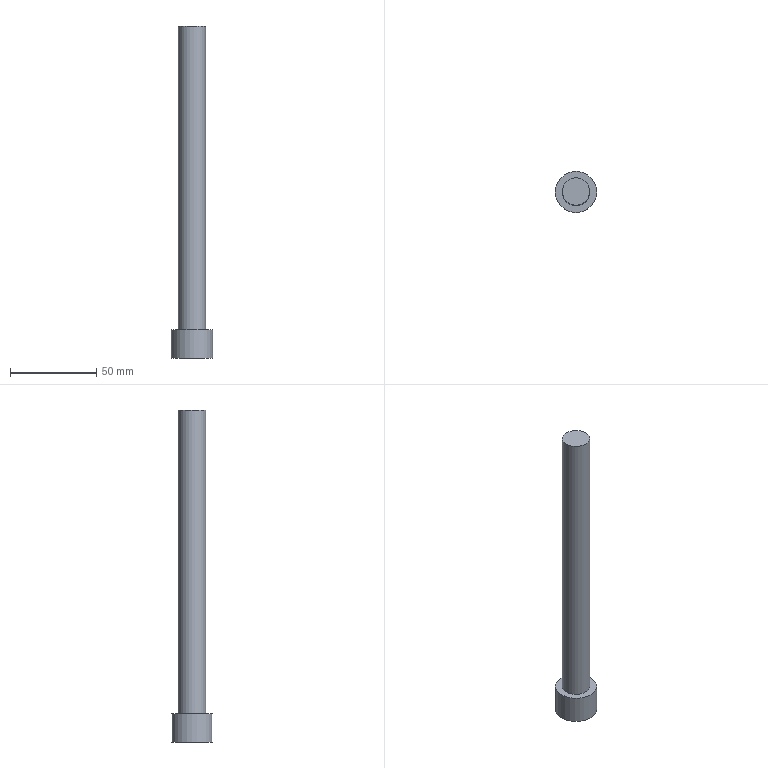Part | NX | features LKM-CI 2 | 1 solid | 12 faces | box 24 x 24 x 193 mm | volume 41551 mm3 | plane 10 | cylinder 2 | commonest cylinder face diameters 16 x1 24 x1
STEP:
#1=CARTESIAN_POINT('',(154.5,89.,-269.5));
#2=VERTEX_POINT('',#1);
#3=CARTESIAN_POINT('',(142.5,89.,-269.5));
#4=DIRECTION('',(0.,0.,1.));
#5=DIRECTION('',(1.,0.,0.));
#6=AXIS2_PLACEMENT_3D('',#3,#4,#5);
#7=CIRCLE('',#6,12.);
#8=EDGE_CURVE('',#2,#2,#7,.T.);
#9=ORIENTED_EDGE('',*,*,#8,.F.);
#10=EDGE_LOOP('',(#9));
#11=FACE_BOUND('',#10,.T.);
#12=CARTESIAN_POINT('',(135.5,84.959,-269.5));
#13=VERTEX_POINT('',#12);
#14=CARTESIAN_POINT('',(142.5,80.917,-269.5));
#15=VERTEX_POINT('',#14);
#16=CARTESIAN_POINT('',(135.5,84.959,-269.5));
#17=DIRECTION('',(0.866,-0.5,0.));
#18=VECTOR('',#17,1000.);
#19=LINE('',#16,#18);
#20=EDGE_CURVE('',#13,#15,#19,.T.);
#21=ORIENTED_EDGE('',*,*,#20,.T.);
#22=CARTESIAN_POINT('',(149.5,84.959,-269.5));
#23=VERTEX_POINT('',#22);
#24=CARTESIAN_POINT('',(142.5,80.917,-269.5));
#25=DIRECTION('',(0.866,0.5,0.));
#26=VECTOR('',#25,1000.);
#27=LINE('',#24,#26);
#28=EDGE_CURVE('',#15,#23,#27,.T.);
#29=ORIENTED_EDGE('',*,*,#28,.T.);
#30=CARTESIAN_POINT('',(149.5,93.041,-269.5));
#31=VERTEX_POINT('',#30);
#32=CARTESIAN_POINT('',(149.5,84.959,-269.5));
#33=DIRECTION('',(0.,1.,0.));
#34=VECTOR('',#33,1000.);
#35=LINE('',#32,#34);
#36=EDGE_CURVE('',#23,#31,#35,.T.);
#37=ORIENTED_EDGE('',*,*,#36,.T.);
#38=CARTESIAN_POINT('',(142.5,97.083,-269.5));
#39=VERTEX_POINT('',#38);
#40=CARTESIAN_POINT('',(149.5,93.041,-269.5));
#41=DIRECTION('',(-0.866,0.5,0.));
#42=VECTOR('',#41,1000.);
#43=LINE('',#40,#42);
#44=EDGE_CURVE('',#31,#39,#43,.T.);
#45=ORIENTED_EDGE('',*,*,#44,.T.);
#46=CARTESIAN_POINT('',(135.5,93.041,-269.5));
#47=VERTEX_POINT('',#46);
#48=CARTESIAN_POINT('',(142.5,97.083,-269.5));
#49=DIRECTION('',(-0.866,-0.5,0.));
#50=VECTOR('',#49,1000.);
#51=LINE('',#48,#50);
#52=EDGE_CURVE('',#39,#47,#51,.T.);
#53=ORIENTED_EDGE('',*,*,#52,.T.);
#54=CARTESIAN_POINT('',(135.5,93.041,-269.5));
#55=DIRECTION('',(0.,-1.,0.));
#56=VECTOR('',#55,1000.);
#57=LINE('',#54,#56);
#58=EDGE_CURVE('',#47,#13,#57,.T.);
#59=ORIENTED_EDGE('',*,*,#58,.T.);
#60=EDGE_LOOP('',(#21,#29,#37,#45,#53,#59));
#61=FACE_BOUND('',#60,.T.);
#62=CARTESIAN_POINT('',(142.5,89.,-269.5));
#63=DIRECTION('',(0.,0.,-1.));
#64=DIRECTION('',(-1.,0.,0.));
#65=AXIS2_PLACEMENT_3D('',#62,#63,#64);
#66=PLANE('',#65);
#67=ADVANCED_FACE('',(#11,#61),#66,.T.);
#68=CARTESIAN_POINT('',(150.5,89.,-76.5));
#69=VERTEX_POINT('',#68);
#70=CARTESIAN_POINT('',(142.5,89.,-76.5));
#71=DIRECTION('',(0.,0.,-1.));
#72=DIRECTION('',(1.,0.,0.));
#73=AXIS2_PLACEMENT_3D('',#70,#71,#72);
#74=CIRCLE('',#73,8.);
#75=EDGE_CURVE('',#69,#69,#74,.T.);
#76=ORIENTED_EDGE('',*,*,#75,.F.);
#77=EDGE_LOOP('',(#76));
#78=FACE_BOUND('',#77,.T.);
#79=CARTESIAN_POINT('',(142.5,89.,-76.5));
#80=DIRECTION('',(0.,0.,1.));
#81=DIRECTION('',(1.,0.,0.));
#82=AXIS2_PLACEMENT_3D('',#79,#80,#81);
#83=PLANE('',#82);
#84=ADVANCED_FACE('',(#78),#83,.T.);
#85=CARTESIAN_POINT('',(150.5,89.,-253.));
#86=VERTEX_POINT('',#85);
#87=CARTESIAN_POINT('',(142.5,89.,-253.));
#88=DIRECTION('',(0.,0.,1.));
#89=DIRECTION('',(1.,0.,0.));
#90=AXIS2_PLACEMENT_3D('',#87,#88,#89);
#91=CIRCLE('',#90,8.);
#92=EDGE_CURVE('',#86,#86,#91,.F.);
#93=ORIENTED_EDGE('',*,*,#92,.F.);
#94=EDGE_LOOP('',(#93));
#95=FACE_BOUND('',#94,.T.);
#96=ORIENTED_EDGE('',*,*,#75,.T.);
#97=EDGE_LOOP('',(#96));
#98=FACE_BOUND('',#97,.T.);
#99=CARTESIAN_POINT('',(142.5,89.,-269.5));
#100=DIRECTION('',(0.,0.,1.));
#101=DIRECTION('',(1.,0.,0.));
#102=AXIS2_PLACEMENT_3D('',#99,#100,#101);
#103=CYLINDRICAL_SURFACE('',#102,8.);
#104=ADVANCED_FACE('',(#95,#98),#103,.T.);
#105=ORIENTED_EDGE('',*,*,#92,.T.);
#106=EDGE_LOOP('',(#105));
#107=FACE_BOUND('',#106,.T.);
#108=CARTESIAN_POINT('',(154.5,89.,-253.));
#109=VERTEX_POINT('',#108);
#110=CARTESIAN_POINT('',(142.5,89.,-253.));
#111=DIRECTION('',(0.,0.,-1.));
#112=DIRECTION('',(1.,0.,0.));
#113=AXIS2_PLACEMENT_3D('',#110,#111,#112);
#114=CIRCLE('',#113,12.);
#115=EDGE_CURVE('',#109,#109,#114,.T.);
#116=ORIENTED_EDGE('',*,*,#115,.F.);
#117=EDGE_LOOP('',(#116));
#118=FACE_BOUND('',#117,.T.);
#119=CARTESIAN_POINT('',(142.5,89.,-253.));
#120=DIRECTION('',(0.,0.,1.));
#121=DIRECTION('',(1.,0.,0.));
#122=AXIS2_PLACEMENT_3D('',#119,#120,#121);
#123=PLANE('',#122);
#124=ADVANCED_FACE('',(#107,#118),#123,.T.);
#125=ORIENTED_EDGE('',*,*,#115,.T.);
#126=EDGE_LOOP('',(#125));
#127=FACE_BOUND('',#126,.T.);
#128=ORIENTED_EDGE('',*,*,#8,.T.);
#129=EDGE_LOOP('',(#128));
#130=FACE_BOUND('',#129,.T.);
#131=CARTESIAN_POINT('',(142.5,89.,-269.5));
#132=DIRECTION('',(0.,0.,1.));
#133=DIRECTION('',(1.,0.,0.));
#134=AXIS2_PLACEMENT_3D('',#131,#132,#133);
#135=CYLINDRICAL_SURFACE('',#134,12.);
#136=ADVANCED_FACE('',(#127,#130),#135,.T.);
#137=CARTESIAN_POINT('',(142.5,80.917,-261.25));
#138=VERTEX_POINT('',#137);
#139=CARTESIAN_POINT('',(135.5,84.959,-261.25));
#140=VERTEX_POINT('',#139);
#141=CARTESIAN_POINT('',(135.5,84.959,-261.25));
#142=DIRECTION('',(0.866,-0.5,0.));
#143=VECTOR('',#142,1000.);
#144=LINE('',#141,#143);
#145=EDGE_CURVE('',#138,#140,#144,.F.);
#146=ORIENTED_EDGE('',*,*,#145,.F.);
#147=CARTESIAN_POINT('',(142.5,80.917,-269.5));
#148=DIRECTION('',(0.,0.,1.));
#149=VECTOR('',#148,1000.);
#150=LINE('',#147,#149);
#151=EDGE_CURVE('',#138,#15,#150,.F.);
#152=ORIENTED_EDGE('',*,*,#151,.T.);
#153=ORIENTED_EDGE('',*,*,#20,.F.);
#154=CARTESIAN_POINT('',(135.5,84.959,-269.5));
#155=DIRECTION('',(0.,0.,1.));
#156=VECTOR('',#155,1000.);
#157=LINE('',#154,#156);
#158=EDGE_CURVE('',#140,#13,#157,.F.);
#159=ORIENTED_EDGE('',*,*,#158,.F.);
#160=EDGE_LOOP('',(#146,#152,#153,#159));
#161=FACE_BOUND('',#160,.T.);
#162=CARTESIAN_POINT('',(139.,82.938,-265.375));
#163=DIRECTION('',(-0.5,-0.866,0.));
#164=DIRECTION('',(0.866,-0.5,0.));
#165=AXIS2_PLACEMENT_3D('',#162,#163,#164);
#166=PLANE('',#165);
#167=ADVANCED_FACE('',(#161),#166,.F.);
#168=CARTESIAN_POINT('',(135.5,93.041,-261.25));
#169=VERTEX_POINT('',#168);
#170=CARTESIAN_POINT('',(135.5,93.041,-261.25));
#171=DIRECTION('',(0.,-1.,0.));
#172=VECTOR('',#171,1000.);
#173=LINE('',#170,#172);
#174=EDGE_CURVE('',#140,#169,#173,.F.);
#175=ORIENTED_EDGE('',*,*,#174,.F.);
#176=ORIENTED_EDGE('',*,*,#158,.T.);
#177=ORIENTED_EDGE('',*,*,#58,.F.);
#178=CARTESIAN_POINT('',(135.5,93.041,-269.5));
#179=DIRECTION('',(0.,0.,1.));
#180=VECTOR('',#179,1000.);
#181=LINE('',#178,#180);
#182=EDGE_CURVE('',#169,#47,#181,.F.);
#183=ORIENTED_EDGE('',*,*,#182,.F.);
#184=EDGE_LOOP('',(#175,#176,#177,#183));
#185=FACE_BOUND('',#184,.T.);
#186=CARTESIAN_POINT('',(135.5,89.,-265.375));
#187=DIRECTION('',(-1.,0.,0.));
#188=DIRECTION('',(0.,0.,1.));
#189=AXIS2_PLACEMENT_3D('',#186,#187,#188);
#190=PLANE('',#189);
#191=ADVANCED_FACE('',(#185),#190,.F.);
#192=CARTESIAN_POINT('',(142.5,97.083,-261.25));
#193=VERTEX_POINT('',#192);
#194=CARTESIAN_POINT('',(142.5,97.083,-261.25));
#195=DIRECTION('',(-0.866,-0.5,0.));
#196=VECTOR('',#195,1000.);
#197=LINE('',#194,#196);
#198=EDGE_CURVE('',#169,#193,#197,.F.);
#199=ORIENTED_EDGE('',*,*,#198,.F.);
#200=ORIENTED_EDGE('',*,*,#182,.T.);
#201=ORIENTED_EDGE('',*,*,#52,.F.);
#202=CARTESIAN_POINT('',(142.5,97.083,-269.5));
#203=DIRECTION('',(0.,0.,1.));
#204=VECTOR('',#203,1000.);
#205=LINE('',#202,#204);
#206=EDGE_CURVE('',#193,#39,#205,.F.);
#207=ORIENTED_EDGE('',*,*,#206,.F.);
#208=EDGE_LOOP('',(#199,#200,#201,#207));
#209=FACE_BOUND('',#208,.T.);
#210=CARTESIAN_POINT('',(139.,95.062,-265.375));
#211=DIRECTION('',(-0.5,0.866,0.));
#212=DIRECTION('',(-0.866,-0.5,0.));
#213=AXIS2_PLACEMENT_3D('',#210,#211,#212);
#214=PLANE('',#213);
#215=ADVANCED_FACE('',(#209),#214,.F.);
#216=CARTESIAN_POINT('',(149.5,93.041,-261.25));
#217=VERTEX_POINT('',#216);
#218=CARTESIAN_POINT('',(149.5,93.041,-261.25));
#219=DIRECTION('',(-0.866,0.5,0.));
#220=VECTOR('',#219,1000.);
#221=LINE('',#218,#220);
#222=EDGE_CURVE('',#193,#217,#221,.F.);
#223=ORIENTED_EDGE('',*,*,#222,.F.);
#224=ORIENTED_EDGE('',*,*,#206,.T.);
#225=ORIENTED_EDGE('',*,*,#44,.F.);
#226=CARTESIAN_POINT('',(149.5,93.041,-269.5));
#227=DIRECTION('',(0.,0.,1.));
#228=VECTOR('',#227,1000.);
#229=LINE('',#226,#228);
#230=EDGE_CURVE('',#217,#31,#229,.F.);
#231=ORIENTED_EDGE('',*,*,#230,.F.);
#232=EDGE_LOOP('',(#223,#224,#225,#231));
#233=FACE_BOUND('',#232,.T.);
#234=CARTESIAN_POINT('',(146.,95.062,-265.375));
#235=DIRECTION('',(0.5,0.866,0.));
#236=DIRECTION('',(-0.866,0.5,0.));
#237=AXIS2_PLACEMENT_3D('',#234,#235,#236);
#238=PLANE('',#237);
#239=ADVANCED_FACE('',(#233),#238,.F.);
#240=CARTESIAN_POINT('',(149.5,84.959,-261.25));
#241=VERTEX_POINT('',#240);
#242=CARTESIAN_POINT('',(149.5,84.959,-261.25));
#243=DIRECTION('',(0.,1.,0.));
#244=VECTOR('',#243,1000.);
#245=LINE('',#242,#244);
#246=EDGE_CURVE('',#217,#241,#245,.F.);
#247=ORIENTED_EDGE('',*,*,#246,.F.);
#248=ORIENTED_EDGE('',*,*,#230,.T.);
#249=ORIENTED_EDGE('',*,*,#36,.F.);
#250=CARTESIAN_POINT('',(149.5,84.959,-269.5));
#251=DIRECTION('',(0.,0.,1.));
#252=VECTOR('',#251,1000.);
#253=LINE('',#250,#252);
#254=EDGE_CURVE('',#241,#23,#253,.F.);
#255=ORIENTED_EDGE('',*,*,#254,.F.);
#256=EDGE_LOOP('',(#247,#248,#249,#255));
#257=FACE_BOUND('',#256,.T.);
#258=CARTESIAN_POINT('',(149.5,89.,-265.375));
#259=DIRECTION('',(1.,0.,0.));
#260=DIRECTION('',(0.,0.,-1.));
#261=AXIS2_PLACEMENT_3D('',#258,#259,#260);
#262=PLANE('',#261);
#263=ADVANCED_FACE('',(#257),#262,.F.);
#264=CARTESIAN_POINT('',(142.5,80.917,-261.25));
#265=DIRECTION('',(0.866,0.5,0.));
#266=VECTOR('',#265,1000.);
#267=LINE('',#264,#266);
#268=EDGE_CURVE('',#241,#138,#267,.F.);
#269=ORIENTED_EDGE('',*,*,#268,.F.);
#270=ORIENTED_EDGE('',*,*,#254,.T.);
#271=ORIENTED_EDGE('',*,*,#28,.F.);
#272=ORIENTED_EDGE('',*,*,#151,.F.);
#273=EDGE_LOOP('',(#269,#270,#271,#272));
#274=FACE_BOUND('',#273,.T.);
#275=CARTESIAN_POINT('',(146.,82.938,-265.375));
#276=DIRECTION('',(0.5,-0.866,0.));
#277=DIRECTION('',(0.866,0.5,0.));
#278=AXIS2_PLACEMENT_3D('',#275,#276,#277);
#279=PLANE('',#278);
#280=ADVANCED_FACE('',(#274),#279,.F.);
#281=ORIENTED_EDGE('',*,*,#174,.T.);
#282=ORIENTED_EDGE('',*,*,#198,.T.);
#283=ORIENTED_EDGE('',*,*,#222,.T.);
#284=ORIENTED_EDGE('',*,*,#246,.T.);
#285=ORIENTED_EDGE('',*,*,#268,.T.);
#286=ORIENTED_EDGE('',*,*,#145,.T.);
#287=EDGE_LOOP('',(#281,#282,#283,#284,#285,#286));
#288=FACE_BOUND('',#287,.T.);
#289=CARTESIAN_POINT('',(142.5,89.,-261.25));
#290=DIRECTION('',(0.,0.,1.));
#291=DIRECTION('',(1.,0.,0.));
#292=AXIS2_PLACEMENT_3D('',#289,#290,#291);
#293=PLANE('',#292);
#294=ADVANCED_FACE('',(#288),#293,.F.);
#295=CLOSED_SHELL('',(#67,#84,#104,#124,#136,#167,#191,#215,#239,#263,#280,#294));
#296=MANIFOLD_SOLID_BREP('',#295);
#297=(LENGTH_UNIT()NAMED_UNIT(*)SI_UNIT(.MILLI.,.METRE.));
#298=UNCERTAINTY_MEASURE_WITH_UNIT(LENGTH_MEASURE(0.00001),#297,'','');
#299=(NAMED_UNIT(*)PLANE_ANGLE_UNIT()SI_UNIT($,.RADIAN.));
#300=(NAMED_UNIT(*)SI_UNIT($,.STERADIAN.)SOLID_ANGLE_UNIT());
#301=(GEOMETRIC_REPRESENTATION_CONTEXT(3)GLOBAL_UNCERTAINTY_ASSIGNED_CONTEXT((#298))GLOBAL_UNIT_ASSIGNED_CONTEXT((#297,#299,#300))REPRESENTATION_CONTEXT('',''));
#302=ADVANCED_BREP_SHAPE_REPRESENTATION('',(#296),#301);